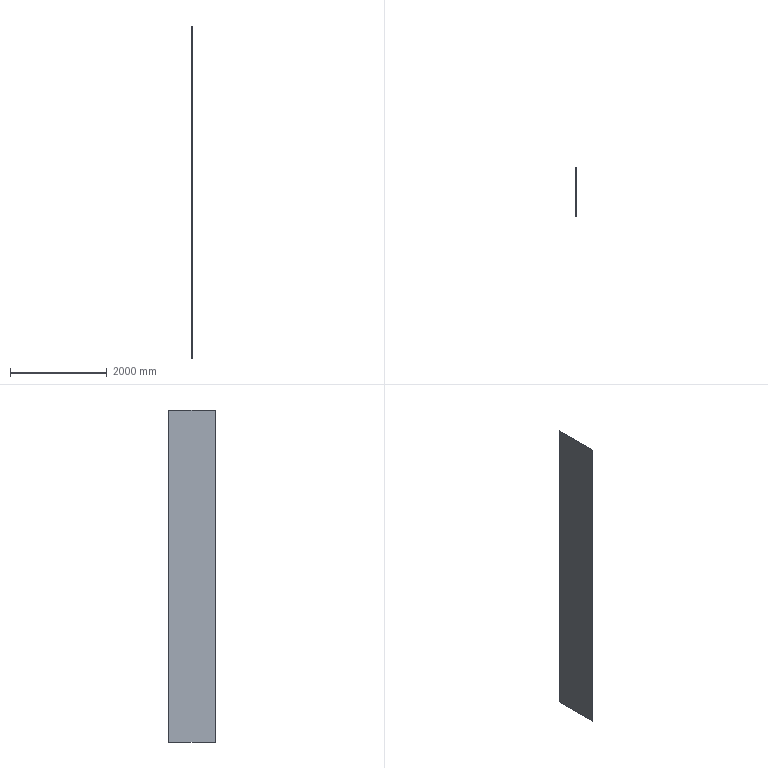Part | SolidWorks | features Fillet 1, FlatPattern 1, SMBaseFlange 1, SheetMetal 1 | 1 solid | 10 faces | box 1.2 x 990 x 6870 mm | volume 8161457 mm3 | plane 6 | cylinder 4 | commonest cylinder face diameters 20 x4
STEP:
#1=CARTESIAN_POINT('',(-1.2,-485.,-3435.));
#2=VERTEX_POINT('',#1);
#3=CARTESIAN_POINT('',(-1.2,485.,-3435.));
#4=VERTEX_POINT('',#3);
#5=CARTESIAN_POINT('',(-1.2,-495.,-3435.));
#6=DIRECTION('',(0.,1.,0.));
#7=VECTOR('',#6,1000.);
#8=LINE('',#5,#7);
#9=EDGE_CURVE('',#2,#4,#8,.T.);
#10=ORIENTED_EDGE('',*,*,#9,.T.);
#11=CARTESIAN_POINT('',(0.,485.,-3435.));
#12=VERTEX_POINT('',#11);
#13=CARTESIAN_POINT('',(-1.2,485.,-3435.));
#14=DIRECTION('',(1.,0.,0.));
#15=VECTOR('',#14,1000.);
#16=LINE('',#13,#15);
#17=EDGE_CURVE('',#4,#12,#16,.T.);
#18=ORIENTED_EDGE('',*,*,#17,.T.);
#19=CARTESIAN_POINT('',(0.,-485.,-3435.));
#20=VERTEX_POINT('',#19);
#21=CARTESIAN_POINT('',(0.,-495.,-3435.));
#22=DIRECTION('',(0.,1.,0.));
#23=VECTOR('',#22,1000.);
#24=LINE('',#21,#23);
#25=EDGE_CURVE('',#20,#12,#24,.T.);
#26=ORIENTED_EDGE('',*,*,#25,.F.);
#27=CARTESIAN_POINT('',(-1.2,-485.,-3435.));
#28=DIRECTION('',(-1.,0.,0.));
#29=VECTOR('',#28,1000.);
#30=LINE('',#27,#29);
#31=EDGE_CURVE('',#20,#2,#30,.T.);
#32=ORIENTED_EDGE('',*,*,#31,.T.);
#33=EDGE_LOOP('',(#10,#18,#26,#32));
#34=FACE_OUTER_BOUND('',#33,.T.);
#35=CARTESIAN_POINT('',(-1.2,-495.,-3435.));
#36=DIRECTION('',(0.,0.,-1.));
#37=DIRECTION('',(-1.,0.,0.));
#38=AXIS2_PLACEMENT_3D('',#35,#36,#37);
#39=PLANE('',#38);
#40=ADVANCED_FACE('',(#34),#39,.T.);
#41=CARTESIAN_POINT('',(-1.2,-495.,3425.));
#42=VERTEX_POINT('',#41);
#43=CARTESIAN_POINT('',(-1.2,-495.,-3425.));
#44=VERTEX_POINT('',#43);
#45=CARTESIAN_POINT('',(-1.2,-495.,3435.));
#46=DIRECTION('',(0.,0.,-1.));
#47=VECTOR('',#46,1000.);
#48=LINE('',#45,#47);
#49=EDGE_CURVE('',#42,#44,#48,.T.);
#50=ORIENTED_EDGE('',*,*,#49,.T.);
#51=CARTESIAN_POINT('',(0.,-495.,-3425.));
#52=VERTEX_POINT('',#51);
#53=CARTESIAN_POINT('',(-1.2,-495.,-3425.));
#54=DIRECTION('',(1.,0.,0.));
#55=VECTOR('',#54,1000.);
#56=LINE('',#53,#55);
#57=EDGE_CURVE('',#44,#52,#56,.T.);
#58=ORIENTED_EDGE('',*,*,#57,.T.);
#59=CARTESIAN_POINT('',(0.,-495.,3425.));
#60=VERTEX_POINT('',#59);
#61=CARTESIAN_POINT('',(0.,-495.,3435.));
#62=DIRECTION('',(0.,0.,-1.));
#63=VECTOR('',#62,1000.);
#64=LINE('',#61,#63);
#65=EDGE_CURVE('',#60,#52,#64,.T.);
#66=ORIENTED_EDGE('',*,*,#65,.F.);
#67=CARTESIAN_POINT('',(-1.2,-495.,3425.));
#68=DIRECTION('',(-1.,0.,0.));
#69=VECTOR('',#68,1000.);
#70=LINE('',#67,#69);
#71=EDGE_CURVE('',#60,#42,#70,.T.);
#72=ORIENTED_EDGE('',*,*,#71,.T.);
#73=EDGE_LOOP('',(#50,#58,#66,#72));
#74=FACE_OUTER_BOUND('',#73,.T.);
#75=CARTESIAN_POINT('',(-1.2,-495.,3435.));
#76=DIRECTION('',(0.,-1.,0.));
#77=DIRECTION('',(0.,0.,-1.));
#78=AXIS2_PLACEMENT_3D('',#75,#76,#77);
#79=PLANE('',#78);
#80=ADVANCED_FACE('',(#74),#79,.T.);
#81=CARTESIAN_POINT('',(0.,485.,3435.));
#82=VERTEX_POINT('',#81);
#83=CARTESIAN_POINT('',(0.,-485.,3435.));
#84=VERTEX_POINT('',#83);
#85=CARTESIAN_POINT('',(0.,-495.,3435.));
#86=DIRECTION('',(0.,-1.,0.));
#87=VECTOR('',#86,1000.);
#88=LINE('',#85,#87);
#89=EDGE_CURVE('',#82,#84,#88,.T.);
#90=ORIENTED_EDGE('',*,*,#89,.F.);
#91=CARTESIAN_POINT('',(-1.2,485.,3435.));
#92=VERTEX_POINT('',#91);
#93=CARTESIAN_POINT('',(-1.2,485.,3435.));
#94=DIRECTION('',(-1.,0.,0.));
#95=VECTOR('',#94,1000.);
#96=LINE('',#93,#95);
#97=EDGE_CURVE('',#82,#92,#96,.T.);
#98=ORIENTED_EDGE('',*,*,#97,.T.);
#99=CARTESIAN_POINT('',(-1.2,-485.,3435.));
#100=VERTEX_POINT('',#99);
#101=CARTESIAN_POINT('',(-1.2,-495.,3435.));
#102=DIRECTION('',(0.,-1.,0.));
#103=VECTOR('',#102,1000.);
#104=LINE('',#101,#103);
#105=EDGE_CURVE('',#92,#100,#104,.T.);
#106=ORIENTED_EDGE('',*,*,#105,.T.);
#107=CARTESIAN_POINT('',(-1.2,-485.,3435.));
#108=DIRECTION('',(1.,0.,0.));
#109=VECTOR('',#108,1000.);
#110=LINE('',#107,#109);
#111=EDGE_CURVE('',#100,#84,#110,.T.);
#112=ORIENTED_EDGE('',*,*,#111,.T.);
#113=EDGE_LOOP('',(#90,#98,#106,#112));
#114=FACE_OUTER_BOUND('',#113,.T.);
#115=CARTESIAN_POINT('',(-1.2,-495.,3435.));
#116=DIRECTION('',(0.,0.,1.));
#117=DIRECTION('',(1.,0.,0.));
#118=AXIS2_PLACEMENT_3D('',#115,#116,#117);
#119=PLANE('',#118);
#120=ADVANCED_FACE('',(#114),#119,.T.);
#121=CARTESIAN_POINT('',(0.,495.,-3425.));
#122=VERTEX_POINT('',#121);
#123=CARTESIAN_POINT('',(0.,495.,3425.));
#124=VERTEX_POINT('',#123);
#125=CARTESIAN_POINT('',(0.,495.,3435.));
#126=DIRECTION('',(0.,0.,1.));
#127=VECTOR('',#126,1000.);
#128=LINE('',#125,#127);
#129=EDGE_CURVE('',#122,#124,#128,.T.);
#130=ORIENTED_EDGE('',*,*,#129,.F.);
#131=CARTESIAN_POINT('',(-1.2,495.,-3425.));
#132=VERTEX_POINT('',#131);
#133=CARTESIAN_POINT('',(-1.2,495.,-3425.));
#134=DIRECTION('',(-1.,0.,0.));
#135=VECTOR('',#134,1000.);
#136=LINE('',#133,#135);
#137=EDGE_CURVE('',#122,#132,#136,.T.);
#138=ORIENTED_EDGE('',*,*,#137,.T.);
#139=CARTESIAN_POINT('',(-1.2,495.,3425.));
#140=VERTEX_POINT('',#139);
#141=CARTESIAN_POINT('',(-1.2,495.,3435.));
#142=DIRECTION('',(0.,0.,1.));
#143=VECTOR('',#142,1000.);
#144=LINE('',#141,#143);
#145=EDGE_CURVE('',#132,#140,#144,.T.);
#146=ORIENTED_EDGE('',*,*,#145,.T.);
#147=CARTESIAN_POINT('',(-1.2,495.,3425.));
#148=DIRECTION('',(1.,0.,0.));
#149=VECTOR('',#148,1000.);
#150=LINE('',#147,#149);
#151=EDGE_CURVE('',#140,#124,#150,.T.);
#152=ORIENTED_EDGE('',*,*,#151,.T.);
#153=EDGE_LOOP('',(#130,#138,#146,#152));
#154=FACE_OUTER_BOUND('',#153,.T.);
#155=CARTESIAN_POINT('',(-1.2,495.,3435.));
#156=DIRECTION('',(0.,1.,0.));
#157=DIRECTION('',(0.,0.,1.));
#158=AXIS2_PLACEMENT_3D('',#155,#156,#157);
#159=PLANE('',#158);
#160=ADVANCED_FACE('',(#154),#159,.T.);
#161=ORIENTED_EDGE('',*,*,#145,.F.);
#162=CARTESIAN_POINT('',(-1.2,485.,-3425.));
#163=DIRECTION('',(-1.,0.,0.));
#164=DIRECTION('',(0.,0.,1.));
#165=AXIS2_PLACEMENT_3D('',#162,#163,#164);
#166=CIRCLE('',#165,10.);
#167=EDGE_CURVE('',#132,#4,#166,.T.);
#168=ORIENTED_EDGE('',*,*,#167,.T.);
#169=ORIENTED_EDGE('',*,*,#9,.F.);
#170=CARTESIAN_POINT('',(-1.2,-485.,-3425.));
#171=DIRECTION('',(-1.,0.,0.));
#172=DIRECTION('',(0.,0.,1.));
#173=AXIS2_PLACEMENT_3D('',#170,#171,#172);
#174=CIRCLE('',#173,10.);
#175=EDGE_CURVE('',#2,#44,#174,.T.);
#176=ORIENTED_EDGE('',*,*,#175,.T.);
#177=ORIENTED_EDGE('',*,*,#49,.F.);
#178=CARTESIAN_POINT('',(-1.2,-485.,3425.));
#179=DIRECTION('',(-1.,0.,0.));
#180=DIRECTION('',(0.,0.,1.));
#181=AXIS2_PLACEMENT_3D('',#178,#179,#180);
#182=CIRCLE('',#181,10.);
#183=EDGE_CURVE('',#42,#100,#182,.T.);
#184=ORIENTED_EDGE('',*,*,#183,.T.);
#185=ORIENTED_EDGE('',*,*,#105,.F.);
#186=CARTESIAN_POINT('',(-1.2,485.,3425.));
#187=DIRECTION('',(-1.,0.,0.));
#188=DIRECTION('',(0.,0.,1.));
#189=AXIS2_PLACEMENT_3D('',#186,#187,#188);
#190=CIRCLE('',#189,10.);
#191=EDGE_CURVE('',#92,#140,#190,.T.);
#192=ORIENTED_EDGE('',*,*,#191,.T.);
#193=EDGE_LOOP('',(#161,#168,#169,#176,#177,#184,#185,#192));
#194=FACE_OUTER_BOUND('',#193,.T.);
#195=CARTESIAN_POINT('',(-1.2,0.,0.));
#196=DIRECTION('',(-1.,0.,0.));
#197=DIRECTION('',(0.,0.,1.));
#198=AXIS2_PLACEMENT_3D('',#195,#196,#197);
#199=PLANE('',#198);
#200=ADVANCED_FACE('',(#194),#199,.T.);
#201=ORIENTED_EDGE('',*,*,#25,.T.);
#202=CARTESIAN_POINT('',(0.,485.,-3425.));
#203=DIRECTION('',(1.,0.,0.));
#204=DIRECTION('',(0.,0.,1.));
#205=AXIS2_PLACEMENT_3D('',#202,#203,#204);
#206=CIRCLE('',#205,10.);
#207=EDGE_CURVE('',#12,#122,#206,.T.);
#208=ORIENTED_EDGE('',*,*,#207,.T.);
#209=ORIENTED_EDGE('',*,*,#129,.T.);
#210=CARTESIAN_POINT('',(0.,485.,3425.));
#211=DIRECTION('',(1.,0.,0.));
#212=DIRECTION('',(0.,0.,1.));
#213=AXIS2_PLACEMENT_3D('',#210,#211,#212);
#214=CIRCLE('',#213,10.);
#215=EDGE_CURVE('',#124,#82,#214,.T.);
#216=ORIENTED_EDGE('',*,*,#215,.T.);
#217=ORIENTED_EDGE('',*,*,#89,.T.);
#218=CARTESIAN_POINT('',(0.,-485.,3425.));
#219=DIRECTION('',(1.,0.,0.));
#220=DIRECTION('',(0.,0.,1.));
#221=AXIS2_PLACEMENT_3D('',#218,#219,#220);
#222=CIRCLE('',#221,10.);
#223=EDGE_CURVE('',#84,#60,#222,.T.);
#224=ORIENTED_EDGE('',*,*,#223,.T.);
#225=ORIENTED_EDGE('',*,*,#65,.T.);
#226=CARTESIAN_POINT('',(0.,-485.,-3425.));
#227=DIRECTION('',(1.,0.,0.));
#228=DIRECTION('',(0.,0.,1.));
#229=AXIS2_PLACEMENT_3D('',#226,#227,#228);
#230=CIRCLE('',#229,10.);
#231=EDGE_CURVE('',#52,#20,#230,.T.);
#232=ORIENTED_EDGE('',*,*,#231,.T.);
#233=EDGE_LOOP('',(#201,#208,#209,#216,#217,#224,#225,#232));
#234=FACE_OUTER_BOUND('',#233,.T.);
#235=CARTESIAN_POINT('',(0.,0.,0.));
#236=DIRECTION('',(-1.,0.,0.));
#237=DIRECTION('',(0.,0.,1.));
#238=AXIS2_PLACEMENT_3D('',#235,#236,#237);
#239=PLANE('',#238);
#240=ADVANCED_FACE('',(#234),#239,.F.);
#241=ORIENTED_EDGE('',*,*,#167,.F.);
#242=ORIENTED_EDGE('',*,*,#137,.F.);
#243=ORIENTED_EDGE('',*,*,#207,.F.);
#244=ORIENTED_EDGE('',*,*,#17,.F.);
#245=EDGE_LOOP('',(#241,#242,#243,#244));
#246=FACE_OUTER_BOUND('',#245,.T.);
#247=CARTESIAN_POINT('',(-1.2,485.,-3425.));
#248=DIRECTION('',(1.,0.,0.));
#249=DIRECTION('',(0.,0.,-1.));
#250=AXIS2_PLACEMENT_3D('',#247,#248,#249);
#251=CYLINDRICAL_SURFACE('',#250,10.);
#252=ADVANCED_FACE('',(#246),#251,.T.);
#253=ORIENTED_EDGE('',*,*,#175,.F.);
#254=ORIENTED_EDGE('',*,*,#31,.F.);
#255=ORIENTED_EDGE('',*,*,#231,.F.);
#256=ORIENTED_EDGE('',*,*,#57,.F.);
#257=EDGE_LOOP('',(#253,#254,#255,#256));
#258=FACE_OUTER_BOUND('',#257,.T.);
#259=CARTESIAN_POINT('',(-1.2,-485.,-3425.));
#260=DIRECTION('',(1.,0.,0.));
#261=DIRECTION('',(0.,0.,-1.));
#262=AXIS2_PLACEMENT_3D('',#259,#260,#261);
#263=CYLINDRICAL_SURFACE('',#262,10.);
#264=ADVANCED_FACE('',(#258),#263,.T.);
#265=ORIENTED_EDGE('',*,*,#191,.F.);
#266=ORIENTED_EDGE('',*,*,#97,.F.);
#267=ORIENTED_EDGE('',*,*,#215,.F.);
#268=ORIENTED_EDGE('',*,*,#151,.F.);
#269=EDGE_LOOP('',(#265,#266,#267,#268));
#270=FACE_OUTER_BOUND('',#269,.T.);
#271=CARTESIAN_POINT('',(-1.2,485.,3425.));
#272=DIRECTION('',(1.,0.,0.));
#273=DIRECTION('',(0.,0.,-1.));
#274=AXIS2_PLACEMENT_3D('',#271,#272,#273);
#275=CYLINDRICAL_SURFACE('',#274,10.);
#276=ADVANCED_FACE('',(#270),#275,.T.);
#277=ORIENTED_EDGE('',*,*,#183,.F.);
#278=ORIENTED_EDGE('',*,*,#71,.F.);
#279=ORIENTED_EDGE('',*,*,#223,.F.);
#280=ORIENTED_EDGE('',*,*,#111,.F.);
#281=EDGE_LOOP('',(#277,#278,#279,#280));
#282=FACE_OUTER_BOUND('',#281,.T.);
#283=CARTESIAN_POINT('',(-1.2,-485.,3425.));
#284=DIRECTION('',(1.,0.,0.));
#285=DIRECTION('',(0.,0.,-1.));
#286=AXIS2_PLACEMENT_3D('',#283,#284,#285);
#287=CYLINDRICAL_SURFACE('',#286,10.);
#288=ADVANCED_FACE('',(#282),#287,.T.);
#289=CLOSED_SHELL('',(#40,#80,#120,#160,#200,#240,#252,#264,#276,#288));
#290=MANIFOLD_SOLID_BREP('',#289);
#291=CARTESIAN_POINT('',(0.,0.,0.));
#292=DIRECTION('',(0.,0.,1.));
#293=DIRECTION('',(1.,0.,0.));
#294=AXIS2_PLACEMENT_3D('',#291,#292,#293);
#295=(LENGTH_UNIT()NAMED_UNIT(*)SI_UNIT(.MILLI.,.METRE.));
#296=UNCERTAINTY_MEASURE_WITH_UNIT(LENGTH_MEASURE(0.00001),#295,'','');
#297=(NAMED_UNIT(*)PLANE_ANGLE_UNIT()SI_UNIT($,.RADIAN.));
#298=(NAMED_UNIT(*)SI_UNIT($,.STERADIAN.)SOLID_ANGLE_UNIT());
#299=(GEOMETRIC_REPRESENTATION_CONTEXT(3)GLOBAL_UNCERTAINTY_ASSIGNED_CONTEXT((#296))GLOBAL_UNIT_ASSIGNED_CONTEXT((#295,#297,#298))REPRESENTATION_CONTEXT('',''));
#300=ADVANCED_BREP_SHAPE_REPRESENTATION('',(#290,#294),#299);